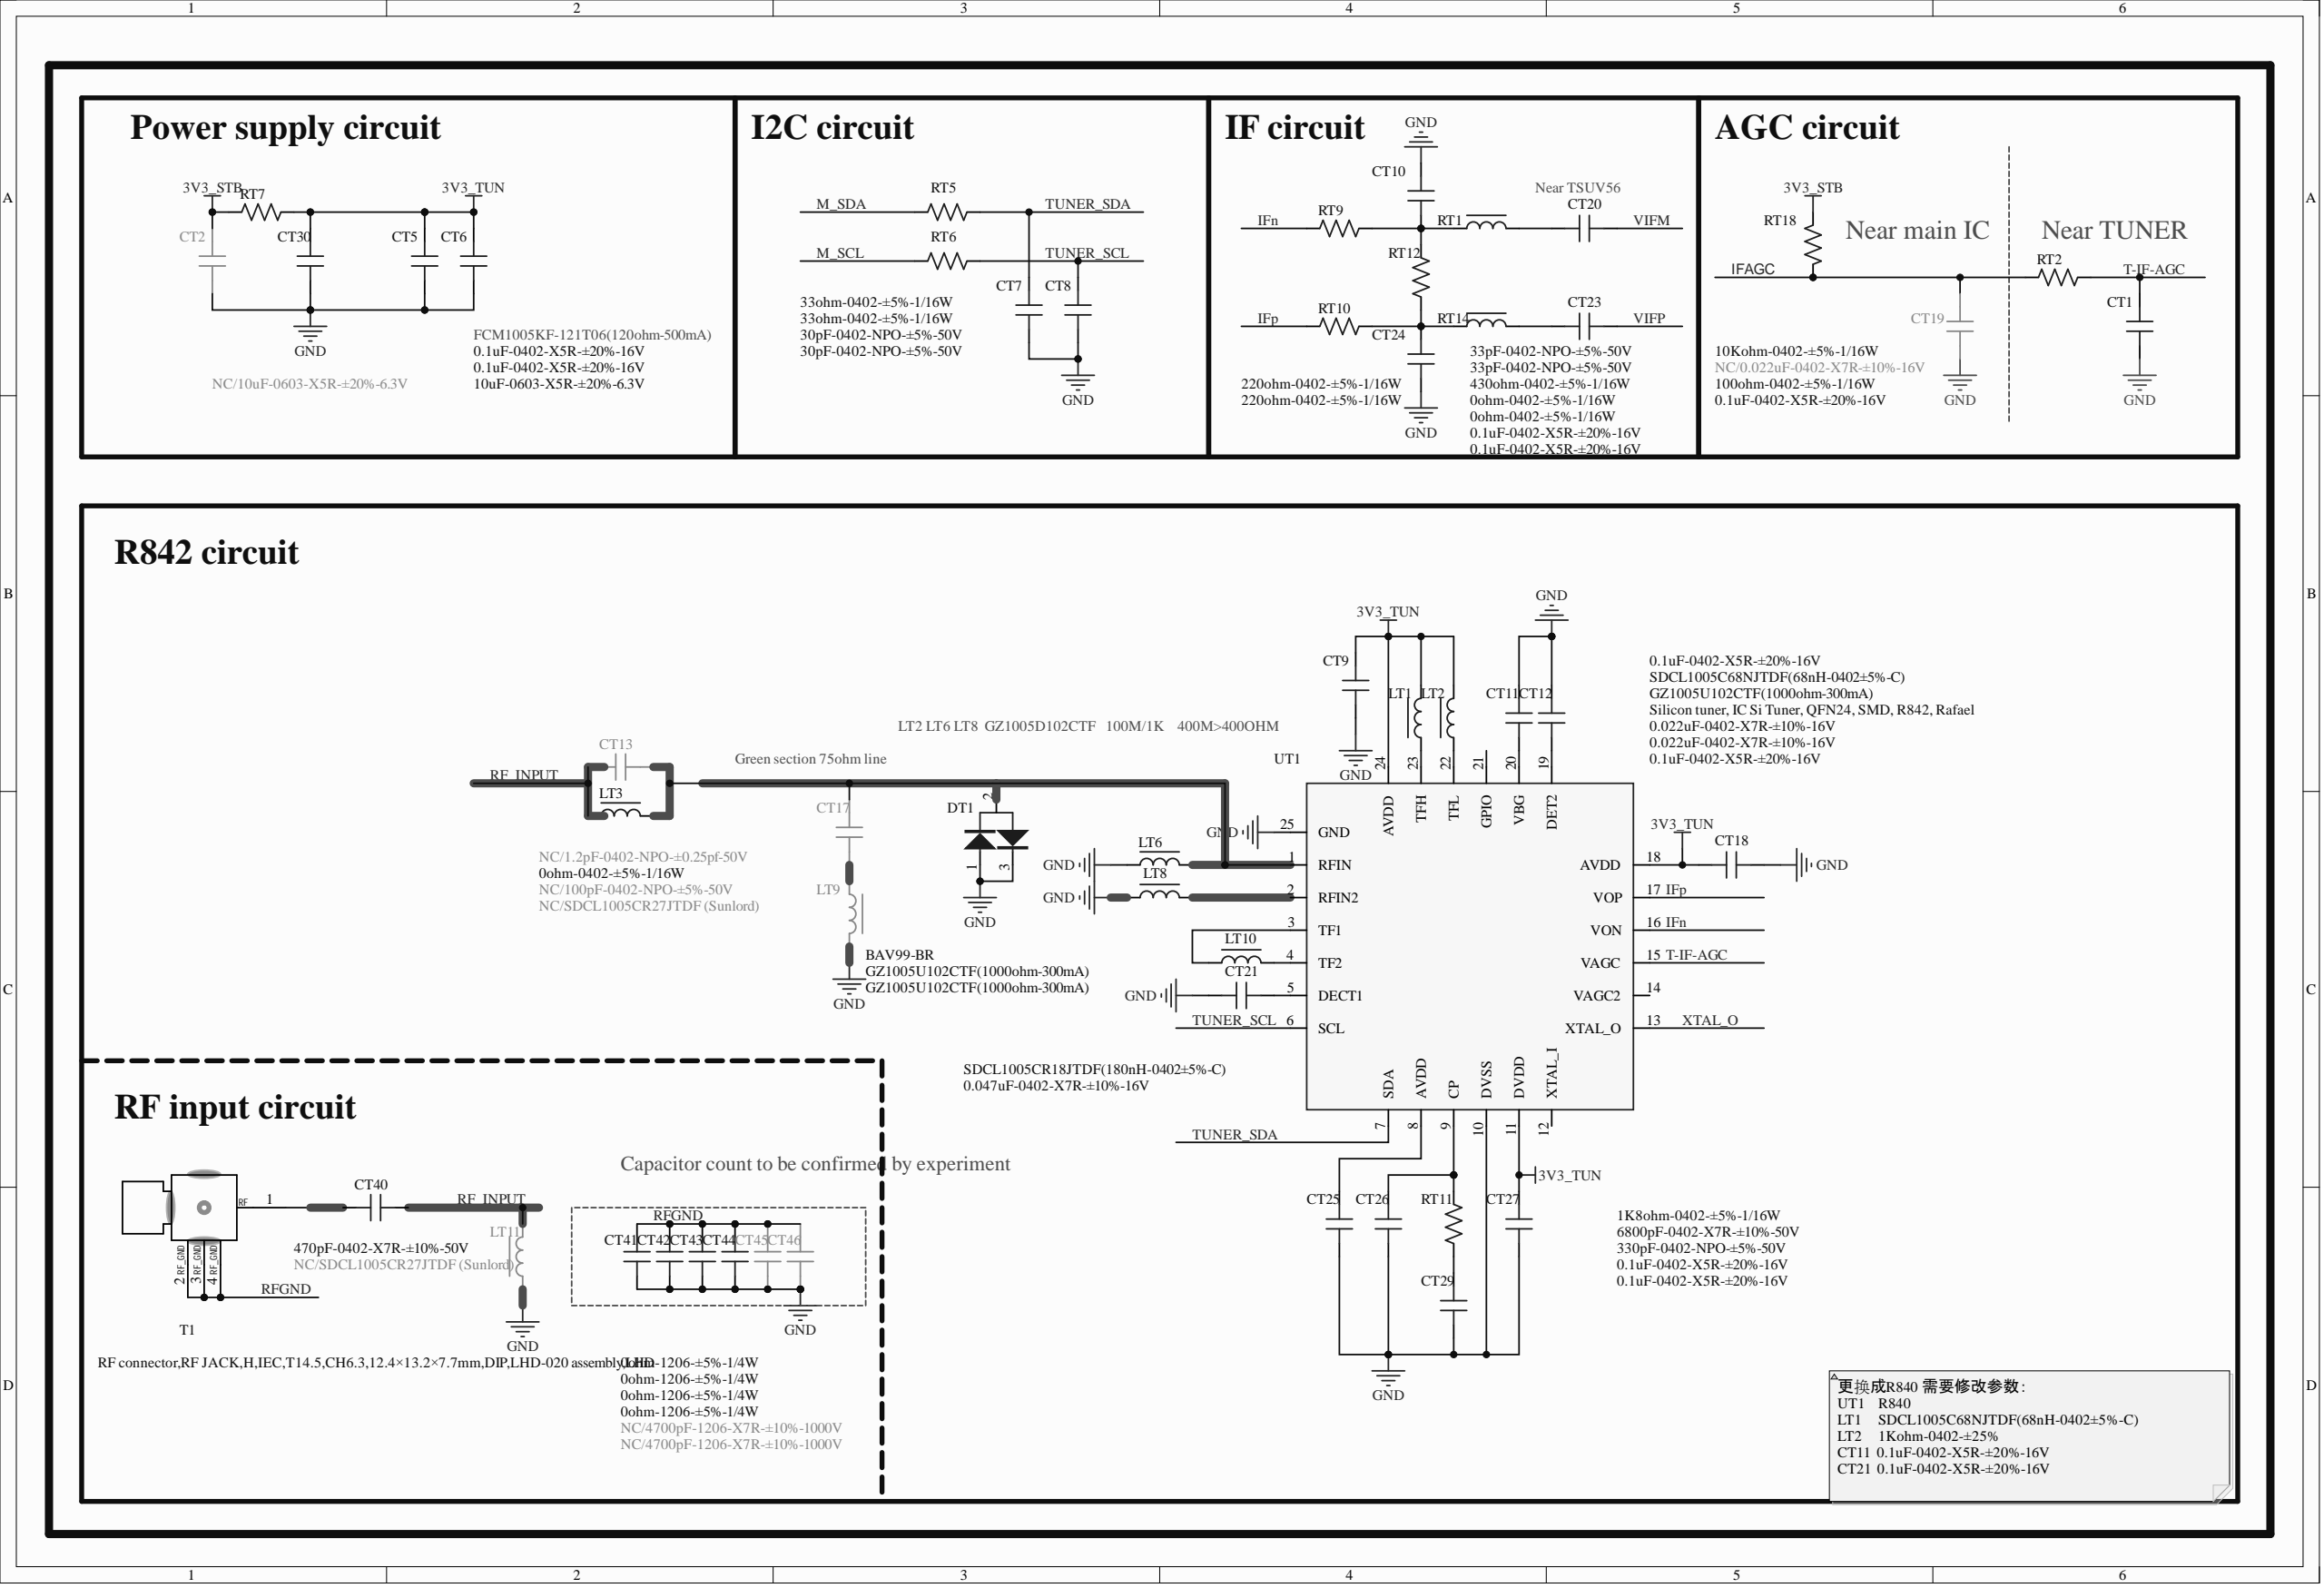Circuit board | Altium Designer | 709 parts | 378 nets | one sheet of the schematic
Parts on this sheet (reference | value | footprint):
CT1 | 0.1uF-0402-X5R-±20%-16V | C0402
CT2 | NC/10uF-0603-X5R-±20%-6.3V | C0603
CT5 | 0.1uF-0402-X5R-±20%-16V | C0402
CT6 | 10uF-0603-X5R-±20%-6.3V | C0603
CT7 | 30pF-0402-NPO-±5%-50V | C0402
CT8 | 30pF-0402-NPO-±5%-50V | C0402
CT9 | 0.1uF-0402-X5R-±20%-16V | C0402
CT10 | 33pF-0402-NPO-±5%-50V | C0402
CT11 | 0.022uF-0402-X7R-±10%-16V | C0402
CT12 | 0.022uF-0402-X7R-±10%-16V | C0402
CT13 | NC/1.2pF-0402-NPO-±0.25pf-50V | C0402
CT17 | NC/100pF-0402-NPO-±5%-50V | C0402
CT18 | 0.1uF-0402-X5R-±20%-16V | C0402
CT19 | NC/0.022uF-0402-X7R-±10%-16V | C0402
CT20 | 0.1uF-0402-X5R-±20%-16V | C0402
CT21 | 0.047uF-0402-X7R-±10%-16V | C0402
CT23 | 0.1uF-0402-X5R-±20%-16V | C0402
CT24 | 33pF-0402-NPO-±5%-50V | C0402
CT25 | 0.1uF-0402-X5R-±20%-16V | C0402
CT26 | 330pF-0402-NPO-±5%-50V | C0402
CT27 | 0.1uF-0402-X5R-±20%-16V | C0402
CT29 | 6800pF-0402-X7R-±10%-50V | C0402
CT30 | 0.1uF-0402-X5R-±20%-16V | C0402
CT40 | 470pF-0402-X7R-±10%-50V | C0402
CT41 | 0ohm-1206-±5%-1/4W | C1206
CT42 | 0ohm-1206-±5%-1/4W | C1206
CT43 | 0ohm-1206-±5%-1/4W | C1206
CT44 | 0ohm-1206-±5%-1/4W | C1206
CT45 | NC/4700pF-1206-X7R-±10%-1000V | C1206
CT46 | NC/4700pF-1206-X7R-±10%-1000V | C1206
DT1 | BAV99-BR | SO-23
LT1 | SDCL1005C68NJTDF(68nH-0402±5%-C) | L0402
LT2 | GZ1005U102CTF(1000ohm-300mA) | L0402
LT3 | 0ohm-0402-±5%-1/16W | L0402
LT6 | GZ1005U102CTF(1000ohm-300mA) | L0402
LT8 | GZ1005U102CTF(1000ohm-300mA) | L0402
LT9 | NC/SDCL1005CR27JTDF (Sunlord) | L0402
LT10 | SDCL1005CR18JTDF(180nH-0402±5%-C) | L0402
LT11 | NC/SDCL1005CR27JTDF (Sunlord) | L0402
RT1 | 0ohm-0402-±5%-1/16W | L0402
RT2 | 100ohm-0402-±5%-1/16W | R0402
RT5 | 33ohm-0402-±5%-1/16W | R0402
RT6 | 33ohm-0402-±5%-1/16W | R0402
RT7 | FCM1005KF-121T06(120ohm-500mA) | R0402
RT9 | 220ohm-0402-±5%-1/16W | R0402
RT10 | 220ohm-0402-±5%-1/16W | R0402
RT11 | 1K8ohm-0402-±5%-1/16W | R0402
RT12 | 430ohm-0402-±5%-1/16W | R0402
RT14 | 0ohm-0402-±5%-1/16W | L0402
RT18 | 10Kohm-0402-±5%-1/16W | R0402
T1 | RF connector,RF JACK,H,IEC,T14.5,CH6.3,12.4×13.2×7.7mm,DIP,LHD-020 assembly,LHD | ANT-IEC14.5-H-短体-NG
UT1 | Silicon tuner, IC Si Tuner, QFN24, SMD, R842, Rafael | QFN24/0.5-3
Nets of these parts (net: part-pin ...):
XTAL_O: UT1-13
VIFP: CT23-2
VIFM: CT20-2
TUNER_SDA: CT7-2 RT5-2 UT1-7
TUNER_SCL: CT8-2 RT6-2 UT1-6
T-IF-AGC: CT1-2 RT2-2 UT1-15
RFGND: CT41-2 CT42-2 CT43-2 CT44-2 CT45-2 CT46-2 T1-2 T1-3 T1-4
RF_INPUT: CT13-1 CT40-2 LT3-1 LT11-1
NetLT10_2: LT10-2 UT1-3
NetLT10_1: LT10-1 UT1-4
NetLT8_1: LT8-1 UT1-2
NetLT2_1: LT2-1 UT1-22
NetLT1_2: LT1-2 UT1-23
NetCT40_1: CT40-1 T1-1
NetCT29_2: CT29-2 RT11-1
NetCT26_2: CT26-2 RT11-2 UT1-9
NetCT25_1: CT25-1 UT1-8
NetCT24_2: CT24-2 RT10-1 RT12-1 RT14-1
NetCT23_1: CT23-1 RT14-2
NetCT21_1: CT21-1 UT1-5
NetCT20_1: CT20-1 RT1-2
NetCT17_1: CT17-1 LT9-2
NetCT13_2: CT13-2 CT17-2 DT1-2 LT3-2 LT6-1 UT1-1
NetCT12_1: CT12-1 UT1-19
NetCT11_2: CT11-2 UT1-20
NetCT10_1: CT10-1 RT1-1 RT9-1 RT12-2
M_SDA: RT5-1
M_SCL: RT6-1
IFp: RT10-2 UT1-17
IFn: RT9-2 UT1-16
IFAGC: CT19-2 RT2-1 RT18-2
GND: CT1-1 CT2-2 CT5-1 CT6-2 CT7-1 CT8-1 CT9-2 CT10-2 CT11-1 CT12-2 CT18-1 CT19-1 CT21-2 CT24-1 CT25-2 CT26-1 CT27-2 CT29-1 CT30-1 CT41-1 CT42-1 CT43-1 CT44-1 CT45-1 CT46-1 DT1-1 DT1-3 LT6-2 LT8-2 LT9-1 LT11-2 UT1-10 UT1-25
3V3_TUN: CT5-2 CT6-1 CT9-1 CT18-2 CT27-1 CT30-2 LT1-1 LT2-2 RT7-2 UT1-11 UT1-18 UT1-24
3V3_STB: CT2-1 RT7-1 RT18-1